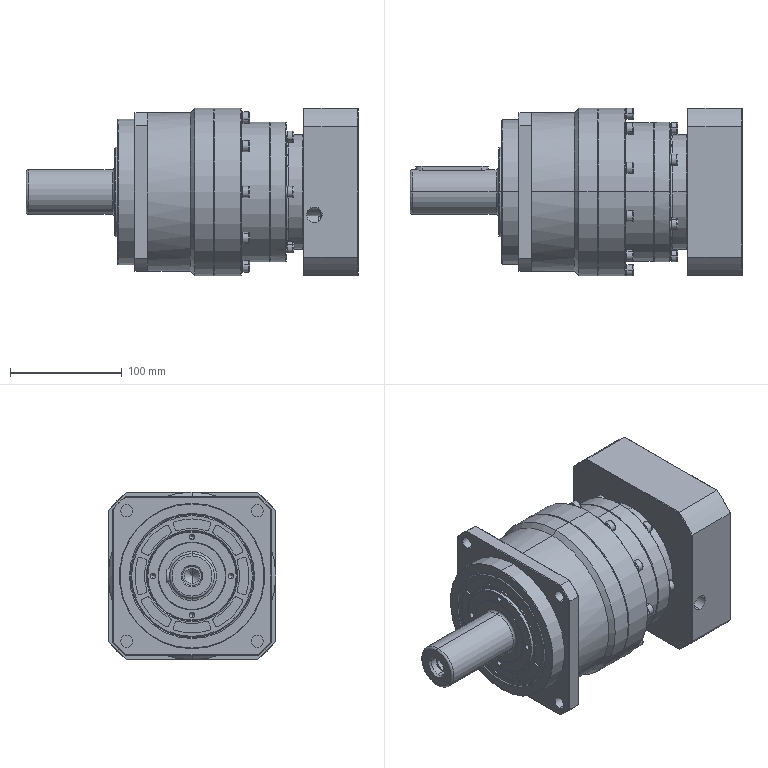Part | SolidWorks | features BaseBody 52 | 52 solids | 1352 faces | box 297 x 150 x 150 mm | volume 3232491 mm3 | plane 585 | cylinder 481 | cone 236 | torus 50 | commonest cylinder face diameters 6.68 x66 9.88 x66 6 x44 6.6 x44 10 x44 4 x40